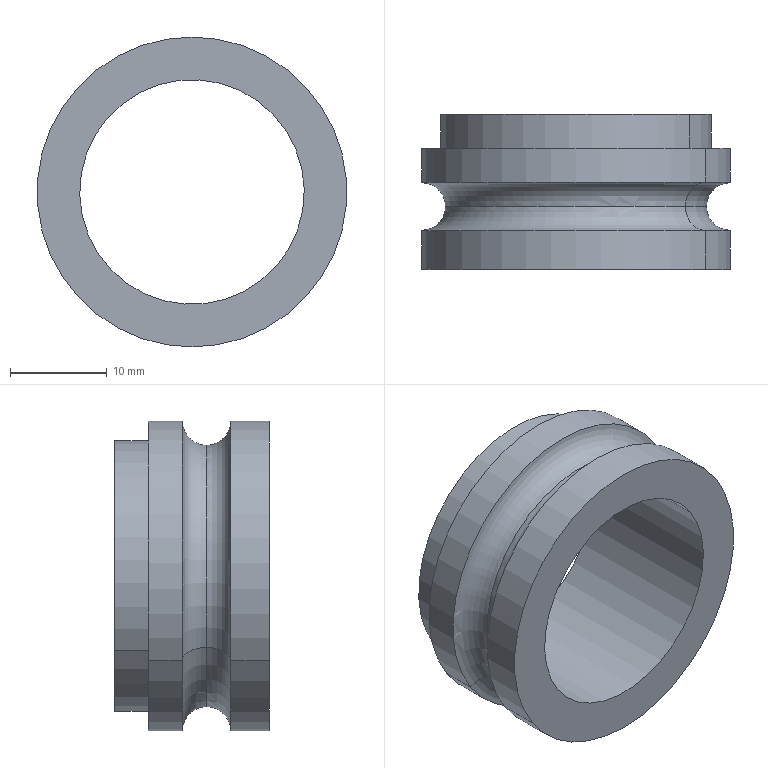Part | SolidWorks | features BaseBody 1 | 1 solid | 15 faces | box 32 x 16 x 32 mm | volume 4523 mm3 | cylinder 8 | torus 4 | plane 3 | commonest cylinder face diameters 32 x4 23.2 x2 28 x2
STEP:
#1=CARTESIAN_POINT('',(259.605,-131.5,280.749));
#2=VERTEX_POINT('',#1);
#3=CARTESIAN_POINT('',(261.698,-129.,282.116));
#4=VERTEX_POINT('',#3);
#5=CARTESIAN_POINT('',(259.605,-129.,280.749));
#6=DIRECTION('',(-0.5469,0.,0.8372));
#7=DIRECTION('',(0.8372,0.,0.5469));
#8=AXIS2_PLACEMENT_3D('',#5,#6,#7);
#9=CIRCLE('',#8,2.5);
#10=EDGE_CURVE('',#2,#4,#9,.T.);
#11=ORIENTED_EDGE('',*,*,#10,.T.);
#12=CARTESIAN_POINT('',(284.302,-129.,296.884));
#13=VERTEX_POINT('',#12);
#14=CARTESIAN_POINT('',(273.,-129.,289.5));
#15=DIRECTION('',(0.,-1.,0.));
#16=DIRECTION('',(0.,0.,-1.));
#17=AXIS2_PLACEMENT_3D('',#14,#15,#16);
#18=CIRCLE('',#17,13.5);
#19=EDGE_CURVE('',#4,#13,#18,.T.);
#20=ORIENTED_EDGE('',*,*,#19,.T.);
#21=CARTESIAN_POINT('',(286.395,-131.5,298.251));
#22=VERTEX_POINT('',#21);
#23=CARTESIAN_POINT('',(286.395,-129.,298.251));
#24=DIRECTION('',(0.5469,0.,-0.8372));
#25=DIRECTION('',(-0.8372,0.,-0.5469));
#26=AXIS2_PLACEMENT_3D('',#23,#24,#25);
#27=CIRCLE('',#26,2.5);
#28=EDGE_CURVE('',#22,#13,#27,.T.);
#29=ORIENTED_EDGE('',*,*,#28,.F.);
#30=CARTESIAN_POINT('',(273.,-131.5,289.5));
#31=DIRECTION('',(0.,1.,0.));
#32=DIRECTION('',(0.,0.,-1.));
#33=AXIS2_PLACEMENT_3D('',#30,#31,#32);
#34=CIRCLE('',#33,16.);
#35=EDGE_CURVE('',#22,#2,#34,.T.);
#36=ORIENTED_EDGE('',*,*,#35,.T.);
#37=EDGE_LOOP('',(#11,#20,#29,#36));
#38=FACE_OUTER_BOUND('',#37,.T.);
#39=CARTESIAN_POINT('',(273.,-129.,289.5));
#40=DIRECTION('',(0.,-1.,0.));
#41=DIRECTION('',(-0.8372,0.,-0.5469));
#42=AXIS2_PLACEMENT_3D('',#39,#40,#41);
#43=TOROIDAL_SURFACE('',#42,16.,2.5);
#44=ADVANCED_FACE('',(#38),#43,.F.);
#45=ORIENTED_EDGE('',*,*,#28,.T.);
#46=CARTESIAN_POINT('',(273.,-129.,289.5));
#47=DIRECTION('',(0.,-1.,0.));
#48=DIRECTION('',(0.,0.,-1.));
#49=AXIS2_PLACEMENT_3D('',#46,#47,#48);
#50=CIRCLE('',#49,13.5);
#51=EDGE_CURVE('',#13,#4,#50,.T.);
#52=ORIENTED_EDGE('',*,*,#51,.T.);
#53=ORIENTED_EDGE('',*,*,#10,.F.);
#54=CARTESIAN_POINT('',(273.,-131.5,289.5));
#55=DIRECTION('',(0.,1.,0.));
#56=DIRECTION('',(0.,0.,-1.));
#57=AXIS2_PLACEMENT_3D('',#54,#55,#56);
#58=CIRCLE('',#57,16.);
#59=EDGE_CURVE('',#2,#22,#58,.T.);
#60=ORIENTED_EDGE('',*,*,#59,.T.);
#61=EDGE_LOOP('',(#45,#52,#53,#60));
#62=FACE_OUTER_BOUND('',#61,.T.);
#63=CARTESIAN_POINT('',(273.,-129.,289.5));
#64=DIRECTION('',(0.,-1.,0.));
#65=DIRECTION('',(-0.8372,0.,-0.5469));
#66=AXIS2_PLACEMENT_3D('',#63,#64,#65);
#67=TOROIDAL_SURFACE('',#66,16.,2.5);
#68=ADVANCED_FACE('',(#62),#67,.F.);
#69=CARTESIAN_POINT('',(286.395,-123.,298.251));
#70=VERTEX_POINT('',#69);
#71=CARTESIAN_POINT('',(259.605,-123.,280.749));
#72=VERTEX_POINT('',#71);
#73=CARTESIAN_POINT('',(273.,-123.,289.5));
#74=DIRECTION('',(0.,1.,0.));
#75=DIRECTION('',(0.,0.,-1.));
#76=AXIS2_PLACEMENT_3D('',#73,#74,#75);
#77=CIRCLE('',#76,16.);
#78=EDGE_CURVE('',#70,#72,#77,.T.);
#79=ORIENTED_EDGE('',*,*,#78,.F.);
#80=CARTESIAN_POINT('',(286.395,-126.5,298.251));
#81=VERTEX_POINT('',#80);
#82=CARTESIAN_POINT('',(286.395,-123.,298.251));
#83=DIRECTION('',(0.,-1.,0.));
#84=VECTOR('',#83,1000.);
#85=LINE('',#82,#84);
#86=EDGE_CURVE('',#70,#81,#85,.T.);
#87=ORIENTED_EDGE('',*,*,#86,.T.);
#88=CARTESIAN_POINT('',(259.605,-126.5,280.749));
#89=VERTEX_POINT('',#88);
#90=CARTESIAN_POINT('',(273.,-126.5,289.5));
#91=DIRECTION('',(0.,-1.,0.));
#92=DIRECTION('',(0.,0.,-1.));
#93=AXIS2_PLACEMENT_3D('',#90,#91,#92);
#94=CIRCLE('',#93,16.);
#95=EDGE_CURVE('',#89,#81,#94,.T.);
#96=ORIENTED_EDGE('',*,*,#95,.F.);
#97=CARTESIAN_POINT('',(259.605,-123.,280.749));
#98=DIRECTION('',(0.,-1.,0.));
#99=VECTOR('',#98,1000.);
#100=LINE('',#97,#99);
#101=EDGE_CURVE('',#72,#89,#100,.T.);
#102=ORIENTED_EDGE('',*,*,#101,.F.);
#103=EDGE_LOOP('',(#79,#87,#96,#102));
#104=FACE_OUTER_BOUND('',#103,.T.);
#105=CARTESIAN_POINT('',(273.,-123.,289.5));
#106=DIRECTION('',(0.,-1.,0.));
#107=DIRECTION('',(-0.8372,0.,-0.5469));
#108=AXIS2_PLACEMENT_3D('',#105,#106,#107);
#109=CYLINDRICAL_SURFACE('',#108,16.);
#110=ADVANCED_FACE('',(#104),#109,.T.);
#111=CARTESIAN_POINT('',(261.28,-119.5,281.843));
#112=VERTEX_POINT('',#111);
#113=CARTESIAN_POINT('',(284.72,-119.5,297.157));
#114=VERTEX_POINT('',#113);
#115=CARTESIAN_POINT('',(273.,-119.5,289.5));
#116=DIRECTION('',(0.,-1.,0.));
#117=DIRECTION('',(0.,0.,-1.));
#118=AXIS2_PLACEMENT_3D('',#115,#116,#117);
#119=CIRCLE('',#118,14.);
#120=EDGE_CURVE('',#112,#114,#119,.T.);
#121=ORIENTED_EDGE('',*,*,#120,.T.);
#122=CARTESIAN_POINT('',(284.72,-123.,297.157));
#123=VERTEX_POINT('',#122);
#124=CARTESIAN_POINT('',(284.72,-119.5,297.157));
#125=DIRECTION('',(0.,-1.,0.));
#126=VECTOR('',#125,1000.);
#127=LINE('',#124,#126);
#128=EDGE_CURVE('',#114,#123,#127,.T.);
#129=ORIENTED_EDGE('',*,*,#128,.T.);
#130=CARTESIAN_POINT('',(261.28,-123.,281.843));
#131=VERTEX_POINT('',#130);
#132=CARTESIAN_POINT('',(273.,-123.,289.5));
#133=DIRECTION('',(0.,-1.,0.));
#134=DIRECTION('',(0.,0.,-1.));
#135=AXIS2_PLACEMENT_3D('',#132,#133,#134);
#136=CIRCLE('',#135,14.);
#137=EDGE_CURVE('',#131,#123,#136,.T.);
#138=ORIENTED_EDGE('',*,*,#137,.F.);
#139=CARTESIAN_POINT('',(261.28,-119.5,281.843));
#140=DIRECTION('',(0.,-1.,0.));
#141=VECTOR('',#140,1000.);
#142=LINE('',#139,#141);
#143=EDGE_CURVE('',#112,#131,#142,.T.);
#144=ORIENTED_EDGE('',*,*,#143,.F.);
#145=EDGE_LOOP('',(#121,#129,#138,#144));
#146=FACE_OUTER_BOUND('',#145,.T.);
#147=CARTESIAN_POINT('',(273.,-119.5,289.5));
#148=DIRECTION('',(0.,-1.,0.));
#149=DIRECTION('',(-0.8372,0.,-0.5469));
#150=AXIS2_PLACEMENT_3D('',#147,#148,#149);
#151=CYLINDRICAL_SURFACE('',#150,14.);
#152=ADVANCED_FACE('',(#146),#151,.T.);
#153=ORIENTED_EDGE('',*,*,#51,.F.);
#154=CARTESIAN_POINT('',(286.395,-129.,298.251));
#155=DIRECTION('',(0.5469,0.,-0.8372));
#156=DIRECTION('',(-0.8372,0.,-0.5469));
#157=AXIS2_PLACEMENT_3D('',#154,#155,#156);
#158=CIRCLE('',#157,2.5);
#159=EDGE_CURVE('',#13,#81,#158,.T.);
#160=ORIENTED_EDGE('',*,*,#159,.T.);
#161=CARTESIAN_POINT('',(273.,-126.5,289.5));
#162=DIRECTION('',(0.,-1.,0.));
#163=DIRECTION('',(0.,0.,-1.));
#164=AXIS2_PLACEMENT_3D('',#161,#162,#163);
#165=CIRCLE('',#164,16.);
#166=EDGE_CURVE('',#81,#89,#165,.T.);
#167=ORIENTED_EDGE('',*,*,#166,.T.);
#168=CARTESIAN_POINT('',(259.605,-129.,280.749));
#169=DIRECTION('',(-0.5469,0.,0.8372));
#170=DIRECTION('',(0.8372,0.,0.5469));
#171=AXIS2_PLACEMENT_3D('',#168,#169,#170);
#172=CIRCLE('',#171,2.5);
#173=EDGE_CURVE('',#4,#89,#172,.T.);
#174=ORIENTED_EDGE('',*,*,#173,.F.);
#175=EDGE_LOOP('',(#153,#160,#167,#174));
#176=FACE_OUTER_BOUND('',#175,.T.);
#177=CARTESIAN_POINT('',(273.,-129.,289.5));
#178=DIRECTION('',(0.,-1.,0.));
#179=DIRECTION('',(-0.8372,0.,-0.5469));
#180=AXIS2_PLACEMENT_3D('',#177,#178,#179);
#181=TOROIDAL_SURFACE('',#180,16.,2.5);
#182=ADVANCED_FACE('',(#176),#181,.F.);
#183=ORIENTED_EDGE('',*,*,#35,.F.);
#184=CARTESIAN_POINT('',(286.395,-135.5,298.251));
#185=VERTEX_POINT('',#184);
#186=CARTESIAN_POINT('',(286.395,-131.5,298.251));
#187=DIRECTION('',(0.,-1.,0.));
#188=VECTOR('',#187,1000.);
#189=LINE('',#186,#188);
#190=EDGE_CURVE('',#22,#185,#189,.T.);
#191=ORIENTED_EDGE('',*,*,#190,.T.);
#192=CARTESIAN_POINT('',(259.605,-135.5,280.749));
#193=VERTEX_POINT('',#192);
#194=CARTESIAN_POINT('',(273.,-135.5,289.5));
#195=DIRECTION('',(0.,-1.,0.));
#196=DIRECTION('',(0.,0.,-1.));
#197=AXIS2_PLACEMENT_3D('',#194,#195,#196);
#198=CIRCLE('',#197,16.);
#199=EDGE_CURVE('',#193,#185,#198,.T.);
#200=ORIENTED_EDGE('',*,*,#199,.F.);
#201=CARTESIAN_POINT('',(259.605,-131.5,280.749));
#202=DIRECTION('',(0.,-1.,0.));
#203=VECTOR('',#202,1000.);
#204=LINE('',#201,#203);
#205=EDGE_CURVE('',#2,#193,#204,.T.);
#206=ORIENTED_EDGE('',*,*,#205,.F.);
#207=EDGE_LOOP('',(#183,#191,#200,#206));
#208=FACE_OUTER_BOUND('',#207,.T.);
#209=CARTESIAN_POINT('',(273.,-131.5,289.5));
#210=DIRECTION('',(0.,-1.,0.));
#211=DIRECTION('',(-0.8372,0.,-0.5469));
#212=AXIS2_PLACEMENT_3D('',#209,#210,#211);
#213=CYLINDRICAL_SURFACE('',#212,16.);
#214=ADVANCED_FACE('',(#208),#213,.T.);
#215=CARTESIAN_POINT('',(263.289,-119.5,283.155));
#216=VERTEX_POINT('',#215);
#217=CARTESIAN_POINT('',(282.711,-119.5,295.845));
#218=VERTEX_POINT('',#217);
#219=CARTESIAN_POINT('',(273.,-119.5,289.5));
#220=DIRECTION('',(0.,1.,0.));
#221=DIRECTION('',(0.,0.,-1.));
#222=AXIS2_PLACEMENT_3D('',#219,#220,#221);
#223=CIRCLE('',#222,11.6);
#224=EDGE_CURVE('',#216,#218,#223,.T.);
#225=ORIENTED_EDGE('',*,*,#224,.T.);
#226=CARTESIAN_POINT('',(282.711,-135.5,295.845));
#227=VERTEX_POINT('',#226);
#228=CARTESIAN_POINT('',(282.711,-119.5,295.845));
#229=DIRECTION('',(0.,-1.,0.));
#230=VECTOR('',#229,1000.);
#231=LINE('',#228,#230);
#232=EDGE_CURVE('',#218,#227,#231,.T.);
#233=ORIENTED_EDGE('',*,*,#232,.T.);
#234=CARTESIAN_POINT('',(263.289,-135.5,283.155));
#235=VERTEX_POINT('',#234);
#236=CARTESIAN_POINT('',(273.,-135.5,289.5));
#237=DIRECTION('',(0.,1.,0.));
#238=DIRECTION('',(0.,0.,-1.));
#239=AXIS2_PLACEMENT_3D('',#236,#237,#238);
#240=CIRCLE('',#239,11.6);
#241=EDGE_CURVE('',#235,#227,#240,.T.);
#242=ORIENTED_EDGE('',*,*,#241,.F.);
#243=CARTESIAN_POINT('',(263.289,-119.5,283.155));
#244=DIRECTION('',(0.,-1.,0.));
#245=VECTOR('',#244,1000.);
#246=LINE('',#243,#245);
#247=EDGE_CURVE('',#216,#235,#246,.T.);
#248=ORIENTED_EDGE('',*,*,#247,.F.);
#249=EDGE_LOOP('',(#225,#233,#242,#248));
#250=FACE_OUTER_BOUND('',#249,.T.);
#251=CARTESIAN_POINT('',(273.,-119.5,289.5));
#252=DIRECTION('',(0.,-1.,0.));
#253=DIRECTION('',(-0.8372,0.,-0.5469));
#254=AXIS2_PLACEMENT_3D('',#251,#252,#253);
#255=CYLINDRICAL_SURFACE('',#254,11.6);
#256=ADVANCED_FACE('',(#250),#255,.F.);
#257=ORIENTED_EDGE('',*,*,#199,.T.);
#258=CARTESIAN_POINT('',(273.,-135.5,289.5));
#259=DIRECTION('',(0.,-1.,0.));
#260=DIRECTION('',(0.,0.,-1.));
#261=AXIS2_PLACEMENT_3D('',#258,#259,#260);
#262=CIRCLE('',#261,16.);
#263=EDGE_CURVE('',#185,#193,#262,.T.);
#264=ORIENTED_EDGE('',*,*,#263,.T.);
#265=EDGE_LOOP('',(#257,#264));
#266=FACE_OUTER_BOUND('',#265,.T.);
#267=ORIENTED_EDGE('',*,*,#241,.T.);
#268=CARTESIAN_POINT('',(273.,-135.5,289.5));
#269=DIRECTION('',(0.,1.,0.));
#270=DIRECTION('',(0.,0.,-1.));
#271=AXIS2_PLACEMENT_3D('',#268,#269,#270);
#272=CIRCLE('',#271,11.6);
#273=EDGE_CURVE('',#227,#235,#272,.T.);
#274=ORIENTED_EDGE('',*,*,#273,.T.);
#275=EDGE_LOOP('',(#267,#274));
#276=FACE_BOUND('',#275,.T.);
#277=CARTESIAN_POINT('',(279.345,-135.5,279.789));
#278=DIRECTION('',(0.,-1.,0.));
#279=DIRECTION('',(0.,0.,-1.));
#280=AXIS2_PLACEMENT_3D('',#277,#278,#279);
#281=PLANE('',#280);
#282=ADVANCED_FACE('',(#266,#276),#281,.T.);
#283=ORIENTED_EDGE('',*,*,#232,.F.);
#284=CARTESIAN_POINT('',(273.,-119.5,289.5));
#285=DIRECTION('',(0.,1.,0.));
#286=DIRECTION('',(0.,0.,-1.));
#287=AXIS2_PLACEMENT_3D('',#284,#285,#286);
#288=CIRCLE('',#287,11.6);
#289=EDGE_CURVE('',#218,#216,#288,.T.);
#290=ORIENTED_EDGE('',*,*,#289,.T.);
#291=ORIENTED_EDGE('',*,*,#247,.T.);
#292=ORIENTED_EDGE('',*,*,#273,.F.);
#293=EDGE_LOOP('',(#283,#290,#291,#292));
#294=FACE_OUTER_BOUND('',#293,.T.);
#295=CARTESIAN_POINT('',(273.,-119.5,289.5));
#296=DIRECTION('',(0.,-1.,0.));
#297=DIRECTION('',(-0.8372,0.,-0.5469));
#298=AXIS2_PLACEMENT_3D('',#295,#296,#297);
#299=CYLINDRICAL_SURFACE('',#298,11.6);
#300=ADVANCED_FACE('',(#294),#299,.F.);
#301=ORIENTED_EDGE('',*,*,#190,.F.);
#302=ORIENTED_EDGE('',*,*,#59,.F.);
#303=ORIENTED_EDGE('',*,*,#205,.T.);
#304=ORIENTED_EDGE('',*,*,#263,.F.);
#305=EDGE_LOOP('',(#301,#302,#303,#304));
#306=FACE_OUTER_BOUND('',#305,.T.);
#307=CARTESIAN_POINT('',(273.,-131.5,289.5));
#308=DIRECTION('',(0.,-1.,0.));
#309=DIRECTION('',(-0.8372,0.,-0.5469));
#310=AXIS2_PLACEMENT_3D('',#307,#308,#309);
#311=CYLINDRICAL_SURFACE('',#310,16.);
#312=ADVANCED_FACE('',(#306),#311,.T.);
#313=ORIENTED_EDGE('',*,*,#120,.F.);
#314=CARTESIAN_POINT('',(273.,-119.5,289.5));
#315=DIRECTION('',(0.,-1.,0.));
#316=DIRECTION('',(0.,0.,-1.));
#317=AXIS2_PLACEMENT_3D('',#314,#315,#316);
#318=CIRCLE('',#317,14.);
#319=EDGE_CURVE('',#114,#112,#318,.T.);
#320=ORIENTED_EDGE('',*,*,#319,.F.);
#321=EDGE_LOOP('',(#313,#320));
#322=FACE_OUTER_BOUND('',#321,.T.);
#323=ORIENTED_EDGE('',*,*,#224,.F.);
#324=ORIENTED_EDGE('',*,*,#289,.F.);
#325=EDGE_LOOP('',(#323,#324));
#326=FACE_BOUND('',#325,.T.);
#327=CARTESIAN_POINT('',(280.657,-119.5,277.78));
#328=DIRECTION('',(0.,-1.,0.));
#329=DIRECTION('',(0.,0.,-1.));
#330=AXIS2_PLACEMENT_3D('',#327,#328,#329);
#331=PLANE('',#330);
#332=ADVANCED_FACE('',(#322,#326),#331,.F.);
#333=ORIENTED_EDGE('',*,*,#19,.F.);
#334=ORIENTED_EDGE('',*,*,#173,.T.);
#335=ORIENTED_EDGE('',*,*,#95,.T.);
#336=ORIENTED_EDGE('',*,*,#159,.F.);
#337=EDGE_LOOP('',(#333,#334,#335,#336));
#338=FACE_OUTER_BOUND('',#337,.T.);
#339=CARTESIAN_POINT('',(273.,-129.,289.5));
#340=DIRECTION('',(0.,-1.,0.));
#341=DIRECTION('',(-0.8372,0.,-0.5469));
#342=AXIS2_PLACEMENT_3D('',#339,#340,#341);
#343=TOROIDAL_SURFACE('',#342,16.,2.5);
#344=ADVANCED_FACE('',(#338),#343,.F.);
#345=ORIENTED_EDGE('',*,*,#128,.F.);
#346=ORIENTED_EDGE('',*,*,#319,.T.);
#347=ORIENTED_EDGE('',*,*,#143,.T.);
#348=CARTESIAN_POINT('',(273.,-123.,289.5));
#349=DIRECTION('',(0.,-1.,0.));
#350=DIRECTION('',(0.,0.,-1.));
#351=AXIS2_PLACEMENT_3D('',#348,#349,#350);
#352=CIRCLE('',#351,14.);
#353=EDGE_CURVE('',#123,#131,#352,.T.);
#354=ORIENTED_EDGE('',*,*,#353,.F.);
#355=EDGE_LOOP('',(#345,#346,#347,#354));
#356=FACE_OUTER_BOUND('',#355,.T.);
#357=CARTESIAN_POINT('',(273.,-119.5,289.5));
#358=DIRECTION('',(0.,-1.,0.));
#359=DIRECTION('',(-0.8372,0.,-0.5469));
#360=AXIS2_PLACEMENT_3D('',#357,#358,#359);
#361=CYLINDRICAL_SURFACE('',#360,14.);
#362=ADVANCED_FACE('',(#356),#361,.T.);
#363=ORIENTED_EDGE('',*,*,#86,.F.);
#364=CARTESIAN_POINT('',(273.,-123.,289.5));
#365=DIRECTION('',(0.,1.,0.));
#366=DIRECTION('',(0.,0.,-1.));
#367=AXIS2_PLACEMENT_3D('',#364,#365,#366);
#368=CIRCLE('',#367,16.);
#369=EDGE_CURVE('',#72,#70,#368,.T.);
#370=ORIENTED_EDGE('',*,*,#369,.F.);
#371=ORIENTED_EDGE('',*,*,#101,.T.);
#372=ORIENTED_EDGE('',*,*,#166,.F.);
#373=EDGE_LOOP('',(#363,#370,#371,#372));
#374=FACE_OUTER_BOUND('',#373,.T.);
#375=CARTESIAN_POINT('',(273.,-123.,289.5));
#376=DIRECTION('',(0.,-1.,0.));
#377=DIRECTION('',(-0.8372,0.,-0.5469));
#378=AXIS2_PLACEMENT_3D('',#375,#376,#377);
#379=CYLINDRICAL_SURFACE('',#378,16.);
#380=ADVANCED_FACE('',(#374),#379,.T.);
#381=ORIENTED_EDGE('',*,*,#369,.T.);
#382=ORIENTED_EDGE('',*,*,#78,.T.);
#383=EDGE_LOOP('',(#381,#382));
#384=FACE_OUTER_BOUND('',#383,.T.);
#385=ORIENTED_EDGE('',*,*,#137,.T.);
#386=ORIENTED_EDGE('',*,*,#353,.T.);
#387=EDGE_LOOP('',(#385,#386));
#388=FACE_BOUND('',#387,.T.);
#389=CARTESIAN_POINT('',(281.751,-123.,276.105));
#390=DIRECTION('',(0.,-1.,0.));
#391=DIRECTION('',(0.,0.,-1.));
#392=AXIS2_PLACEMENT_3D('',#389,#390,#391);
#393=PLANE('',#392);
#394=ADVANCED_FACE('',(#384,#388),#393,.F.);
#395=CLOSED_SHELL('',(#44,#68,#110,#152,#182,#214,#256,#282,#300,#312,#332,#344,#362,#380,#394));
#396=MANIFOLD_SOLID_BREP('',#395);
#397=CARTESIAN_POINT('',(0.,0.,0.));
#398=DIRECTION('',(0.,0.,1.));
#399=DIRECTION('',(1.,0.,0.));
#400=AXIS2_PLACEMENT_3D('',#397,#398,#399);
#401=(LENGTH_UNIT()NAMED_UNIT(*)SI_UNIT(.MILLI.,.METRE.));
#402=UNCERTAINTY_MEASURE_WITH_UNIT(LENGTH_MEASURE(0.00001),#401,'','');
#403=(NAMED_UNIT(*)PLANE_ANGLE_UNIT()SI_UNIT($,.RADIAN.));
#404=(NAMED_UNIT(*)SI_UNIT($,.STERADIAN.)SOLID_ANGLE_UNIT());
#405=(GEOMETRIC_REPRESENTATION_CONTEXT(3)GLOBAL_UNCERTAINTY_ASSIGNED_CONTEXT((#402))GLOBAL_UNIT_ASSIGNED_CONTEXT((#401,#403,#404))REPRESENTATION_CONTEXT('',''));
#406=ADVANCED_BREP_SHAPE_REPRESENTATION('',(#396,#400),#405);